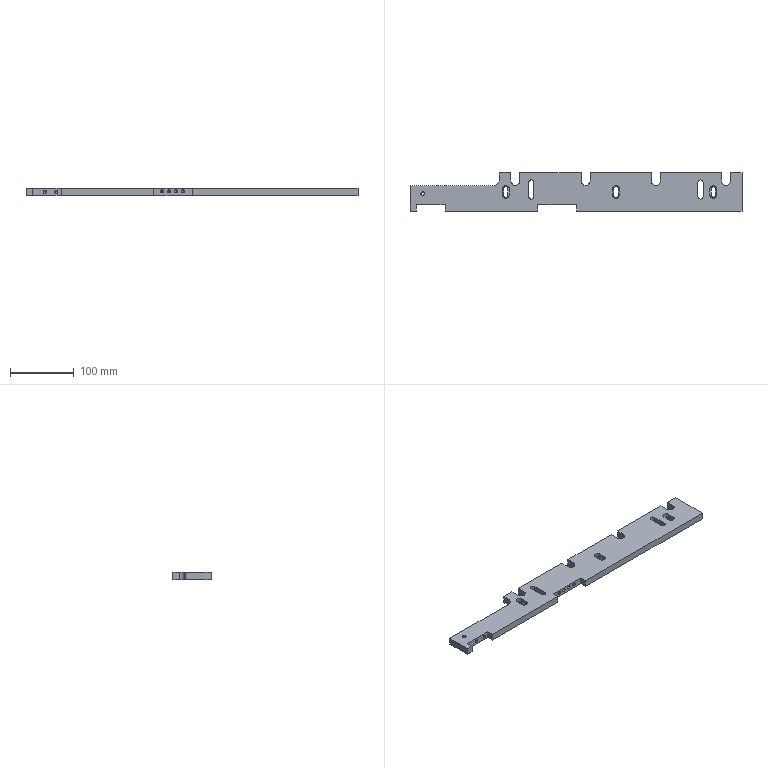Part | STEP file | Tube feed_id954_x_t | 1 solid | 94 faces | box 520 x 59.75 x 11 mm | volume 276450 mm3 | plane 49 | cylinder 28 | cone 17 | commonest cylinder face diameters 4.2 x6 6.8 x6 10.5 x6 8 x4 14 x4 5 x1